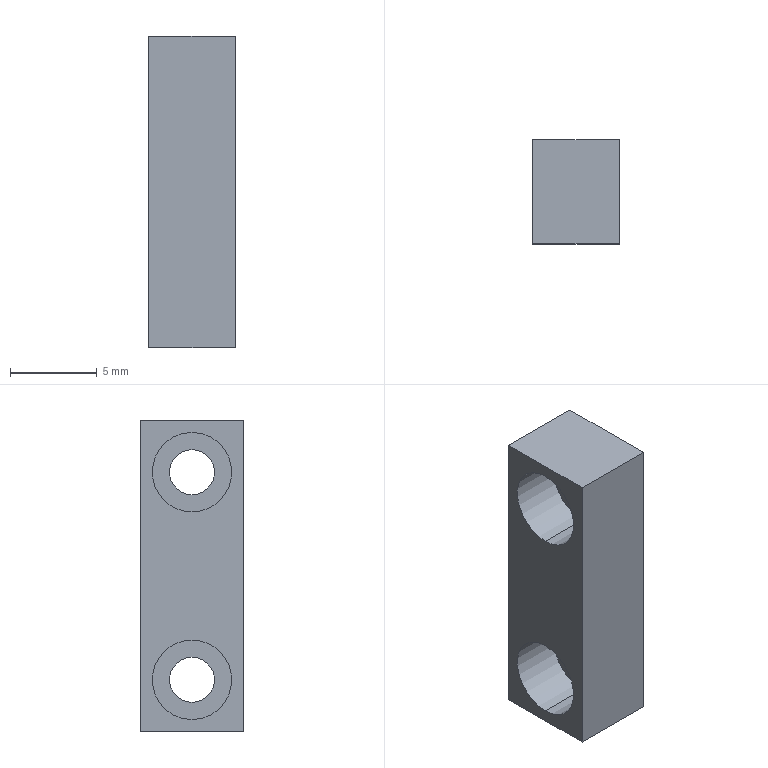Part | SolidWorks | features Cut 1, Extrusion 1, ICE 1 | 1 solid | 16 faces | box 5 x 6 x 18 mm | volume 419.049 mm3 | cylinder 8 | plane 8 | commonest cylinder face diameters 2.6 x4 4.6 x4
STEP:
#1=CARTESIAN_POINT('',(0.5,3.,3.7));
#2=VERTEX_POINT('',#1);
#3=CARTESIAN_POINT('',(0.5,3.,8.3));
#4=VERTEX_POINT('',#3);
#5=CARTESIAN_POINT('',(0.5,3.,6.));
#6=DIRECTION('',(-1.,0.,0.));
#7=DIRECTION('',(0.,0.,1.));
#8=AXIS2_PLACEMENT_3D('',#5,#6,#7);
#9=CIRCLE('',#8,2.3);
#10=EDGE_CURVE('',#2,#4,#9,.T.);
#11=ORIENTED_EDGE('',*,*,#10,.F.);
#12=CARTESIAN_POINT('',(-2.5,3.,3.7));
#13=VERTEX_POINT('',#12);
#14=CARTESIAN_POINT('',(0.5,3.,3.7));
#15=DIRECTION('',(-1.,0.,0.));
#16=VECTOR('',#15,1000.);
#17=LINE('',#14,#16);
#18=EDGE_CURVE('',#2,#13,#17,.T.);
#19=ORIENTED_EDGE('',*,*,#18,.T.);
#20=CARTESIAN_POINT('',(-2.5,3.,8.3));
#21=VERTEX_POINT('',#20);
#22=CARTESIAN_POINT('',(-2.5,3.,6.));
#23=DIRECTION('',(-1.,0.,0.));
#24=DIRECTION('',(0.,0.,1.));
#25=AXIS2_PLACEMENT_3D('',#22,#23,#24);
#26=CIRCLE('',#25,2.3);
#27=EDGE_CURVE('',#13,#21,#26,.T.);
#28=ORIENTED_EDGE('',*,*,#27,.T.);
#29=CARTESIAN_POINT('',(0.5,3.,8.3));
#30=DIRECTION('',(-1.,0.,0.));
#31=VECTOR('',#30,1000.);
#32=LINE('',#29,#31);
#33=EDGE_CURVE('',#4,#21,#32,.T.);
#34=ORIENTED_EDGE('',*,*,#33,.F.);
#35=EDGE_LOOP('',(#11,#19,#28,#34));
#36=FACE_OUTER_BOUND('',#35,.T.);
#37=CARTESIAN_POINT('',(0.5,3.,6.));
#38=DIRECTION('',(-1.,0.,0.));
#39=DIRECTION('',(0.,0.,1.));
#40=AXIS2_PLACEMENT_3D('',#37,#38,#39);
#41=CYLINDRICAL_SURFACE('',#40,2.3);
#42=ADVANCED_FACE('',(#36),#41,.F.);
#43=CARTESIAN_POINT('',(0.5,3.,-8.3));
#44=VERTEX_POINT('',#43);
#45=CARTESIAN_POINT('',(0.5,3.,-3.7));
#46=VERTEX_POINT('',#45);
#47=CARTESIAN_POINT('',(0.5,3.,-6.));
#48=DIRECTION('',(-1.,0.,0.));
#49=DIRECTION('',(0.,0.,1.));
#50=AXIS2_PLACEMENT_3D('',#47,#48,#49);
#51=CIRCLE('',#50,2.3);
#52=EDGE_CURVE('',#44,#46,#51,.T.);
#53=ORIENTED_EDGE('',*,*,#52,.F.);
#54=CARTESIAN_POINT('',(-2.5,3.,-8.3));
#55=VERTEX_POINT('',#54);
#56=CARTESIAN_POINT('',(0.5,3.,-8.3));
#57=DIRECTION('',(-1.,0.,0.));
#58=VECTOR('',#57,1000.);
#59=LINE('',#56,#58);
#60=EDGE_CURVE('',#44,#55,#59,.T.);
#61=ORIENTED_EDGE('',*,*,#60,.T.);
#62=CARTESIAN_POINT('',(-2.5,3.,-3.7));
#63=VERTEX_POINT('',#62);
#64=CARTESIAN_POINT('',(-2.5,3.,-6.));
#65=DIRECTION('',(-1.,0.,0.));
#66=DIRECTION('',(0.,0.,1.));
#67=AXIS2_PLACEMENT_3D('',#64,#65,#66);
#68=CIRCLE('',#67,2.3);
#69=EDGE_CURVE('',#55,#63,#68,.T.);
#70=ORIENTED_EDGE('',*,*,#69,.T.);
#71=CARTESIAN_POINT('',(0.5,3.,-3.7));
#72=DIRECTION('',(-1.,0.,0.));
#73=VECTOR('',#72,1000.);
#74=LINE('',#71,#73);
#75=EDGE_CURVE('',#46,#63,#74,.T.);
#76=ORIENTED_EDGE('',*,*,#75,.F.);
#77=EDGE_LOOP('',(#53,#61,#70,#76));
#78=FACE_OUTER_BOUND('',#77,.T.);
#79=CARTESIAN_POINT('',(0.5,3.,-6.));
#80=DIRECTION('',(-1.,0.,0.));
#81=DIRECTION('',(0.,0.,1.));
#82=AXIS2_PLACEMENT_3D('',#79,#80,#81);
#83=CYLINDRICAL_SURFACE('',#82,2.3);
#84=ADVANCED_FACE('',(#78),#83,.F.);
#85=CARTESIAN_POINT('',(2.5,3.,-7.3));
#86=VERTEX_POINT('',#85);
#87=CARTESIAN_POINT('',(2.5,3.,-4.7));
#88=VERTEX_POINT('',#87);
#89=CARTESIAN_POINT('',(2.5,3.,-6.));
#90=DIRECTION('',(-1.,0.,0.));
#91=DIRECTION('',(0.,0.,1.));
#92=AXIS2_PLACEMENT_3D('',#89,#90,#91);
#93=CIRCLE('',#92,1.3);
#94=EDGE_CURVE('',#86,#88,#93,.T.);
#95=ORIENTED_EDGE('',*,*,#94,.F.);
#96=CARTESIAN_POINT('',(0.5,3.,-7.3));
#97=VERTEX_POINT('',#96);
#98=CARTESIAN_POINT('',(7.5,3.,-7.3));
#99=DIRECTION('',(-1.,0.,0.));
#100=VECTOR('',#99,1000.);
#101=LINE('',#98,#100);
#102=EDGE_CURVE('',#86,#97,#101,.T.);
#103=ORIENTED_EDGE('',*,*,#102,.T.);
#104=CARTESIAN_POINT('',(0.5,3.,-4.7));
#105=VERTEX_POINT('',#104);
#106=CARTESIAN_POINT('',(0.5,3.,-6.));
#107=DIRECTION('',(1.,0.,0.));
#108=DIRECTION('',(0.,0.,1.));
#109=AXIS2_PLACEMENT_3D('',#106,#107,#108);
#110=CIRCLE('',#109,1.3);
#111=EDGE_CURVE('',#105,#97,#110,.T.);
#112=ORIENTED_EDGE('',*,*,#111,.F.);
#113=CARTESIAN_POINT('',(7.5,3.,-4.7));
#114=DIRECTION('',(-1.,0.,0.));
#115=VECTOR('',#114,1000.);
#116=LINE('',#113,#115);
#117=EDGE_CURVE('',#88,#105,#116,.T.);
#118=ORIENTED_EDGE('',*,*,#117,.F.);
#119=EDGE_LOOP('',(#95,#103,#112,#118));
#120=FACE_OUTER_BOUND('',#119,.T.);
#121=CARTESIAN_POINT('',(7.5,3.,-6.));
#122=DIRECTION('',(-1.,0.,0.));
#123=DIRECTION('',(0.,0.,1.));
#124=AXIS2_PLACEMENT_3D('',#121,#122,#123);
#125=CYLINDRICAL_SURFACE('',#124,1.3);
#126=ADVANCED_FACE('',(#120),#125,.F.);
#127=CARTESIAN_POINT('',(2.5,3.,4.7));
#128=VERTEX_POINT('',#127);
#129=CARTESIAN_POINT('',(2.5,3.,7.3));
#130=VERTEX_POINT('',#129);
#131=CARTESIAN_POINT('',(2.5,3.,6.));
#132=DIRECTION('',(-1.,0.,0.));
#133=DIRECTION('',(0.,0.,1.));
#134=AXIS2_PLACEMENT_3D('',#131,#132,#133);
#135=CIRCLE('',#134,1.3);
#136=EDGE_CURVE('',#128,#130,#135,.T.);
#137=ORIENTED_EDGE('',*,*,#136,.F.);
#138=CARTESIAN_POINT('',(0.5,3.,4.7));
#139=VERTEX_POINT('',#138);
#140=CARTESIAN_POINT('',(7.5,3.,4.7));
#141=DIRECTION('',(-1.,0.,0.));
#142=VECTOR('',#141,1000.);
#143=LINE('',#140,#142);
#144=EDGE_CURVE('',#128,#139,#143,.T.);
#145=ORIENTED_EDGE('',*,*,#144,.T.);
#146=CARTESIAN_POINT('',(0.5,3.,7.3));
#147=VERTEX_POINT('',#146);
#148=CARTESIAN_POINT('',(0.5,3.,6.));
#149=DIRECTION('',(1.,0.,0.));
#150=DIRECTION('',(0.,0.,1.));
#151=AXIS2_PLACEMENT_3D('',#148,#149,#150);
#152=CIRCLE('',#151,1.3);
#153=EDGE_CURVE('',#147,#139,#152,.T.);
#154=ORIENTED_EDGE('',*,*,#153,.F.);
#155=CARTESIAN_POINT('',(7.5,3.,7.3));
#156=DIRECTION('',(-1.,0.,0.));
#157=VECTOR('',#156,1000.);
#158=LINE('',#155,#157);
#159=EDGE_CURVE('',#130,#147,#158,.T.);
#160=ORIENTED_EDGE('',*,*,#159,.F.);
#161=EDGE_LOOP('',(#137,#145,#154,#160));
#162=FACE_OUTER_BOUND('',#161,.T.);
#163=CARTESIAN_POINT('',(7.5,3.,6.));
#164=DIRECTION('',(-1.,0.,0.));
#165=DIRECTION('',(0.,0.,1.));
#166=AXIS2_PLACEMENT_3D('',#163,#164,#165);
#167=CYLINDRICAL_SURFACE('',#166,1.3);
#168=ADVANCED_FACE('',(#162),#167,.F.);
#169=ORIENTED_EDGE('',*,*,#144,.F.);
#170=CARTESIAN_POINT('',(2.5,3.,6.));
#171=DIRECTION('',(-1.,0.,0.));
#172=DIRECTION('',(0.,0.,1.));
#173=AXIS2_PLACEMENT_3D('',#170,#171,#172);
#174=CIRCLE('',#173,1.3);
#175=EDGE_CURVE('',#130,#128,#174,.T.);
#176=ORIENTED_EDGE('',*,*,#175,.F.);
#177=ORIENTED_EDGE('',*,*,#159,.T.);
#178=CARTESIAN_POINT('',(0.5,3.,6.));
#179=DIRECTION('',(1.,0.,0.));
#180=DIRECTION('',(0.,0.,1.));
#181=AXIS2_PLACEMENT_3D('',#178,#179,#180);
#182=CIRCLE('',#181,1.3);
#183=EDGE_CURVE('',#139,#147,#182,.T.);
#184=ORIENTED_EDGE('',*,*,#183,.F.);
#185=EDGE_LOOP('',(#169,#176,#177,#184));
#186=FACE_OUTER_BOUND('',#185,.T.);
#187=CARTESIAN_POINT('',(7.5,3.,6.));
#188=DIRECTION('',(-1.,0.,0.));
#189=DIRECTION('',(0.,0.,1.));
#190=AXIS2_PLACEMENT_3D('',#187,#188,#189);
#191=CYLINDRICAL_SURFACE('',#190,1.3);
#192=ADVANCED_FACE('',(#186),#191,.F.);
#193=ORIENTED_EDGE('',*,*,#102,.F.);
#194=CARTESIAN_POINT('',(2.5,3.,-6.));
#195=DIRECTION('',(-1.,0.,0.));
#196=DIRECTION('',(0.,0.,1.));
#197=AXIS2_PLACEMENT_3D('',#194,#195,#196);
#198=CIRCLE('',#197,1.3);
#199=EDGE_CURVE('',#88,#86,#198,.T.);
#200=ORIENTED_EDGE('',*,*,#199,.F.);
#201=ORIENTED_EDGE('',*,*,#117,.T.);
#202=CARTESIAN_POINT('',(0.5,3.,-6.));
#203=DIRECTION('',(1.,0.,0.));
#204=DIRECTION('',(0.,0.,1.));
#205=AXIS2_PLACEMENT_3D('',#202,#203,#204);
#206=CIRCLE('',#205,1.3);
#207=EDGE_CURVE('',#97,#105,#206,.T.);
#208=ORIENTED_EDGE('',*,*,#207,.F.);
#209=EDGE_LOOP('',(#193,#200,#201,#208));
#210=FACE_OUTER_BOUND('',#209,.T.);
#211=CARTESIAN_POINT('',(7.5,3.,-6.));
#212=DIRECTION('',(-1.,0.,0.));
#213=DIRECTION('',(0.,0.,1.));
#214=AXIS2_PLACEMENT_3D('',#211,#212,#213);
#215=CYLINDRICAL_SURFACE('',#214,1.3);
#216=ADVANCED_FACE('',(#210),#215,.F.);
#217=ORIENTED_EDGE('',*,*,#199,.T.);
#218=ORIENTED_EDGE('',*,*,#94,.T.);
#219=EDGE_LOOP('',(#217,#218));
#220=FACE_BOUND('',#219,.T.);
#221=ORIENTED_EDGE('',*,*,#175,.T.);
#222=ORIENTED_EDGE('',*,*,#136,.T.);
#223=EDGE_LOOP('',(#221,#222));
#224=FACE_BOUND('',#223,.T.);
#225=CARTESIAN_POINT('',(2.5,0.,9.));
#226=VERTEX_POINT('',#225);
#227=CARTESIAN_POINT('',(2.5,0.,-9.));
#228=VERTEX_POINT('',#227);
#229=CARTESIAN_POINT('',(2.5,0.,-9.));
#230=DIRECTION('',(0.,0.,-1.));
#231=VECTOR('',#230,1000.);
#232=LINE('',#229,#231);
#233=EDGE_CURVE('',#226,#228,#232,.T.);
#234=ORIENTED_EDGE('',*,*,#233,.T.);
#235=CARTESIAN_POINT('',(2.5,6.,-9.));
#236=VERTEX_POINT('',#235);
#237=CARTESIAN_POINT('',(2.5,6.,-9.));
#238=DIRECTION('',(0.,-1.,0.));
#239=VECTOR('',#238,1000.);
#240=LINE('',#237,#239);
#241=EDGE_CURVE('',#236,#228,#240,.T.);
#242=ORIENTED_EDGE('',*,*,#241,.F.);
#243=CARTESIAN_POINT('',(2.5,6.,9.));
#244=VERTEX_POINT('',#243);
#245=CARTESIAN_POINT('',(2.5,6.,-9.));
#246=DIRECTION('',(0.,0.,-1.));
#247=VECTOR('',#246,1000.);
#248=LINE('',#245,#247);
#249=EDGE_CURVE('',#244,#236,#248,.T.);
#250=ORIENTED_EDGE('',*,*,#249,.F.);
#251=CARTESIAN_POINT('',(2.5,6.,9.));
#252=DIRECTION('',(0.,-1.,0.));
#253=VECTOR('',#252,1000.);
#254=LINE('',#251,#253);
#255=EDGE_CURVE('',#244,#226,#254,.T.);
#256=ORIENTED_EDGE('',*,*,#255,.T.);
#257=EDGE_LOOP('',(#234,#242,#250,#256));
#258=FACE_OUTER_BOUND('',#257,.T.);
#259=CARTESIAN_POINT('',(2.5,6.,-9.));
#260=DIRECTION('',(-1.,0.,0.));
#261=DIRECTION('',(0.,0.,1.));
#262=AXIS2_PLACEMENT_3D('',#259,#260,#261);
#263=PLANE('',#262);
#264=ADVANCED_FACE('',(#220,#224,#258),#263,.F.);
#265=CARTESIAN_POINT('',(-2.5,0.,-9.));
#266=VERTEX_POINT('',#265);
#267=CARTESIAN_POINT('',(-2.5,0.,-9.));
#268=DIRECTION('',(-1.,0.,0.));
#269=VECTOR('',#268,1000.);
#270=LINE('',#267,#269);
#271=EDGE_CURVE('',#228,#266,#270,.T.);
#272=ORIENTED_EDGE('',*,*,#271,.T.);
#273=CARTESIAN_POINT('',(-2.5,6.,-9.));
#274=VERTEX_POINT('',#273);
#275=CARTESIAN_POINT('',(-2.5,6.,-9.));
#276=DIRECTION('',(0.,-1.,0.));
#277=VECTOR('',#276,1000.);
#278=LINE('',#275,#277);
#279=EDGE_CURVE('',#274,#266,#278,.T.);
#280=ORIENTED_EDGE('',*,*,#279,.F.);
#281=CARTESIAN_POINT('',(-2.5,6.,-9.));
#282=DIRECTION('',(-1.,0.,0.));
#283=VECTOR('',#282,1000.);
#284=LINE('',#281,#283);
#285=EDGE_CURVE('',#236,#274,#284,.T.);
#286=ORIENTED_EDGE('',*,*,#285,.F.);
#287=ORIENTED_EDGE('',*,*,#241,.T.);
#288=EDGE_LOOP('',(#272,#280,#286,#287));
#289=FACE_OUTER_BOUND('',#288,.T.);
#290=CARTESIAN_POINT('',(-2.5,6.,-9.));
#291=DIRECTION('',(0.,0.,1.));
#292=DIRECTION('',(1.,0.,0.));
#293=AXIS2_PLACEMENT_3D('',#290,#291,#292);
#294=PLANE('',#293);
#295=ADVANCED_FACE('',(#289),#294,.F.);
#296=CARTESIAN_POINT('',(-2.5,3.,6.));
#297=DIRECTION('',(-1.,0.,0.));
#298=DIRECTION('',(0.,0.,1.));
#299=AXIS2_PLACEMENT_3D('',#296,#297,#298);
#300=CIRCLE('',#299,2.3);
#301=EDGE_CURVE('',#21,#13,#300,.T.);
#302=ORIENTED_EDGE('',*,*,#301,.F.);
#303=ORIENTED_EDGE('',*,*,#27,.F.);
#304=EDGE_LOOP('',(#302,#303));
#305=FACE_BOUND('',#304,.T.);
#306=CARTESIAN_POINT('',(-2.5,3.,-6.));
#307=DIRECTION('',(-1.,0.,0.));
#308=DIRECTION('',(0.,0.,1.));
#309=AXIS2_PLACEMENT_3D('',#306,#307,#308);
#310=CIRCLE('',#309,2.3);
#311=EDGE_CURVE('',#63,#55,#310,.T.);
#312=ORIENTED_EDGE('',*,*,#311,.F.);
#313=ORIENTED_EDGE('',*,*,#69,.F.);
#314=EDGE_LOOP('',(#312,#313));
#315=FACE_BOUND('',#314,.T.);
#316=CARTESIAN_POINT('',(-2.5,0.,9.));
#317=VERTEX_POINT('',#316);
#318=CARTESIAN_POINT('',(-2.5,0.,-9.));
#319=DIRECTION('',(0.,0.,1.));
#320=VECTOR('',#319,1000.);
#321=LINE('',#318,#320);
#322=EDGE_CURVE('',#266,#317,#321,.T.);
#323=ORIENTED_EDGE('',*,*,#322,.T.);
#324=CARTESIAN_POINT('',(-2.5,6.,9.));
#325=VERTEX_POINT('',#324);
#326=CARTESIAN_POINT('',(-2.5,6.,9.));
#327=DIRECTION('',(0.,-1.,0.));
#328=VECTOR('',#327,1000.);
#329=LINE('',#326,#328);
#330=EDGE_CURVE('',#325,#317,#329,.T.);
#331=ORIENTED_EDGE('',*,*,#330,.F.);
#332=CARTESIAN_POINT('',(-2.5,6.,-9.));
#333=DIRECTION('',(0.,0.,1.));
#334=VECTOR('',#333,1000.);
#335=LINE('',#332,#334);
#336=EDGE_CURVE('',#274,#325,#335,.T.);
#337=ORIENTED_EDGE('',*,*,#336,.F.);
#338=ORIENTED_EDGE('',*,*,#279,.T.);
#339=EDGE_LOOP('',(#323,#331,#337,#338));
#340=FACE_OUTER_BOUND('',#339,.T.);
#341=CARTESIAN_POINT('',(-2.5,6.,-9.));
#342=DIRECTION('',(1.,0.,0.));
#343=DIRECTION('',(0.,0.,-1.));
#344=AXIS2_PLACEMENT_3D('',#341,#342,#343);
#345=PLANE('',#344);
#346=ADVANCED_FACE('',(#305,#315,#340),#345,.F.);
#347=CARTESIAN_POINT('',(-2.5,0.,9.));
#348=DIRECTION('',(1.,0.,0.));
#349=VECTOR('',#348,1000.);
#350=LINE('',#347,#349);
#351=EDGE_CURVE('',#317,#226,#350,.T.);
#352=ORIENTED_EDGE('',*,*,#351,.T.);
#353=ORIENTED_EDGE('',*,*,#255,.F.);
#354=CARTESIAN_POINT('',(-2.5,6.,9.));
#355=DIRECTION('',(1.,0.,0.));
#356=VECTOR('',#355,1000.);
#357=LINE('',#354,#356);
#358=EDGE_CURVE('',#325,#244,#357,.T.);
#359=ORIENTED_EDGE('',*,*,#358,.F.);
#360=ORIENTED_EDGE('',*,*,#330,.T.);
#361=EDGE_LOOP('',(#352,#353,#359,#360));
#362=FACE_OUTER_BOUND('',#361,.T.);
#363=CARTESIAN_POINT('',(-2.5,6.,9.));
#364=DIRECTION('',(0.,0.,-1.));
#365=DIRECTION('',(-1.,0.,0.));
#366=AXIS2_PLACEMENT_3D('',#363,#364,#365);
#367=PLANE('',#366);
#368=ADVANCED_FACE('',(#362),#367,.F.);
#369=ORIENTED_EDGE('',*,*,#249,.T.);
#370=ORIENTED_EDGE('',*,*,#285,.T.);
#371=ORIENTED_EDGE('',*,*,#336,.T.);
#372=ORIENTED_EDGE('',*,*,#358,.T.);
#373=EDGE_LOOP('',(#369,#370,#371,#372));
#374=FACE_OUTER_BOUND('',#373,.T.);
#375=CARTESIAN_POINT('',(0.,6.,0.));
#376=DIRECTION('',(0.,1.,0.));
#377=DIRECTION('',(0.,0.,1.));
#378=AXIS2_PLACEMENT_3D('',#375,#376,#377);
#379=PLANE('',#378);
#380=ADVANCED_FACE('',(#374),#379,.T.);
#381=ORIENTED_EDGE('',*,*,#233,.F.);
#382=ORIENTED_EDGE('',*,*,#351,.F.);
#383=ORIENTED_EDGE('',*,*,#322,.F.);
#384=ORIENTED_EDGE('',*,*,#271,.F.);
#385=EDGE_LOOP('',(#381,#382,#383,#384));
#386=FACE_OUTER_BOUND('',#385,.T.);
#387=CARTESIAN_POINT('',(0.,0.,0.));
#388=DIRECTION('',(0.,1.,0.));
#389=DIRECTION('',(0.,0.,1.));
#390=AXIS2_PLACEMENT_3D('',#387,#388,#389);
#391=PLANE('',#390);
#392=ADVANCED_FACE('',(#386),#391,.F.);
#393=CARTESIAN_POINT('',(0.5,3.,-6.));
#394=DIRECTION('',(-1.,0.,0.));
#395=DIRECTION('',(0.,0.,1.));
#396=AXIS2_PLACEMENT_3D('',#393,#394,#395);
#397=CIRCLE('',#396,2.3);
#398=EDGE_CURVE('',#46,#44,#397,.T.);
#399=ORIENTED_EDGE('',*,*,#398,.T.);
#400=ORIENTED_EDGE('',*,*,#52,.T.);
#401=EDGE_LOOP('',(#399,#400));
#402=FACE_OUTER_BOUND('',#401,.T.);
#403=ORIENTED_EDGE('',*,*,#111,.T.);
#404=ORIENTED_EDGE('',*,*,#207,.T.);
#405=EDGE_LOOP('',(#403,#404));
#406=FACE_BOUND('',#405,.T.);
#407=CARTESIAN_POINT('',(0.5,3.,-6.));
#408=DIRECTION('',(-1.,0.,0.));
#409=DIRECTION('',(0.,0.,1.));
#410=AXIS2_PLACEMENT_3D('',#407,#408,#409);
#411=PLANE('',#410);
#412=ADVANCED_FACE('',(#402,#406),#411,.T.);
#413=ORIENTED_EDGE('',*,*,#60,.F.);
#414=ORIENTED_EDGE('',*,*,#398,.F.);
#415=ORIENTED_EDGE('',*,*,#75,.T.);
#416=ORIENTED_EDGE('',*,*,#311,.T.);
#417=EDGE_LOOP('',(#413,#414,#415,#416));
#418=FACE_OUTER_BOUND('',#417,.T.);
#419=CARTESIAN_POINT('',(0.5,3.,-6.));
#420=DIRECTION('',(-1.,0.,0.));
#421=DIRECTION('',(0.,0.,1.));
#422=AXIS2_PLACEMENT_3D('',#419,#420,#421);
#423=CYLINDRICAL_SURFACE('',#422,2.3);
#424=ADVANCED_FACE('',(#418),#423,.F.);
#425=CARTESIAN_POINT('',(0.5,3.,6.));
#426=DIRECTION('',(-1.,0.,0.));
#427=DIRECTION('',(0.,0.,1.));
#428=AXIS2_PLACEMENT_3D('',#425,#426,#427);
#429=CIRCLE('',#428,2.3);
#430=EDGE_CURVE('',#4,#2,#429,.T.);
#431=ORIENTED_EDGE('',*,*,#430,.T.);
#432=ORIENTED_EDGE('',*,*,#10,.T.);
#433=EDGE_LOOP('',(#431,#432));
#434=FACE_OUTER_BOUND('',#433,.T.);
#435=ORIENTED_EDGE('',*,*,#153,.T.);
#436=ORIENTED_EDGE('',*,*,#183,.T.);
#437=EDGE_LOOP('',(#435,#436));
#438=FACE_BOUND('',#437,.T.);
#439=CARTESIAN_POINT('',(0.5,3.,6.));
#440=DIRECTION('',(-1.,0.,0.));
#441=DIRECTION('',(0.,0.,1.));
#442=AXIS2_PLACEMENT_3D('',#439,#440,#441);
#443=PLANE('',#442);
#444=ADVANCED_FACE('',(#434,#438),#443,.T.);
#445=ORIENTED_EDGE('',*,*,#18,.F.);
#446=ORIENTED_EDGE('',*,*,#430,.F.);
#447=ORIENTED_EDGE('',*,*,#33,.T.);
#448=ORIENTED_EDGE('',*,*,#301,.T.);
#449=EDGE_LOOP('',(#445,#446,#447,#448));
#450=FACE_OUTER_BOUND('',#449,.T.);
#451=CARTESIAN_POINT('',(0.5,3.,6.));
#452=DIRECTION('',(-1.,0.,0.));
#453=DIRECTION('',(0.,0.,1.));
#454=AXIS2_PLACEMENT_3D('',#451,#452,#453);
#455=CYLINDRICAL_SURFACE('',#454,2.3);
#456=ADVANCED_FACE('',(#450),#455,.F.);
#457=CLOSED_SHELL('',(#42,#84,#126,#168,#192,#216,#264,#295,#346,#368,#380,#392,#412,#424,#444,#456));
#458=MANIFOLD_SOLID_BREP('',#457);
#459=CARTESIAN_POINT('',(0.,0.,0.));
#460=DIRECTION('',(0.,0.,1.));
#461=DIRECTION('',(1.,0.,0.));
#462=AXIS2_PLACEMENT_3D('',#459,#460,#461);
#463=(LENGTH_UNIT()NAMED_UNIT(*)SI_UNIT(.MILLI.,.METRE.));
#464=UNCERTAINTY_MEASURE_WITH_UNIT(LENGTH_MEASURE(0.00001),#463,'','');
#465=(NAMED_UNIT(*)PLANE_ANGLE_UNIT()SI_UNIT($,.RADIAN.));
#466=(NAMED_UNIT(*)SI_UNIT($,.STERADIAN.)SOLID_ANGLE_UNIT());
#467=(GEOMETRIC_REPRESENTATION_CONTEXT(3)GLOBAL_UNCERTAINTY_ASSIGNED_CONTEXT((#464))GLOBAL_UNIT_ASSIGNED_CONTEXT((#463,#465,#466))REPRESENTATION_CONTEXT('',''));
#468=ADVANCED_BREP_SHAPE_REPRESENTATION('',(#458,#462),#467);